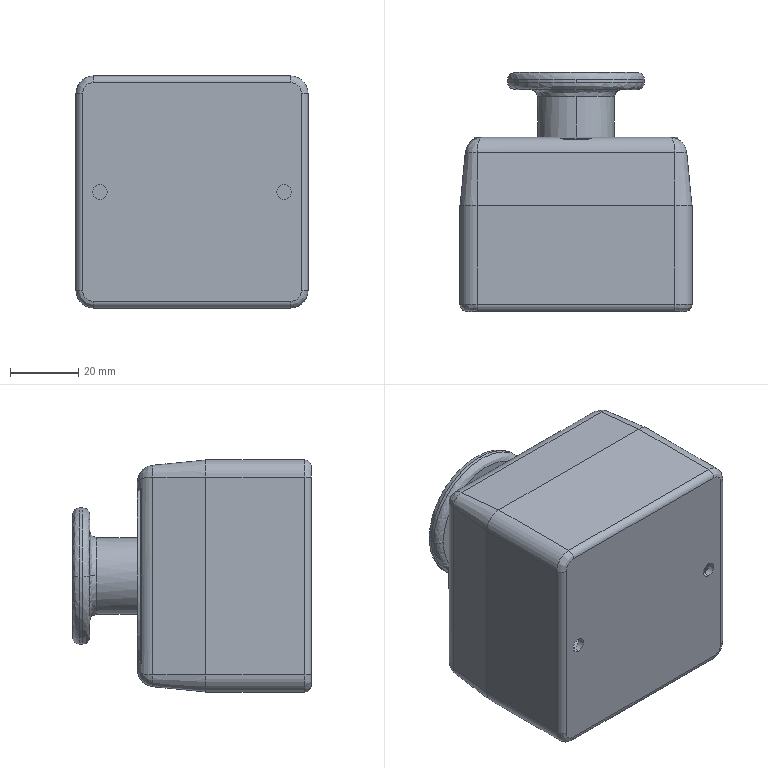Part | STEP file | stop_-005 | 1 solid | 449 faces | box 68 x 70 x 68 mm | volume 54810 mm3 | plane 376 | cylinder 43 | spline 22 | cone 8 | commonest cylinder face diameters 6 x8 10 x8 60 x5 1 x4 4 x4 4.3 x4